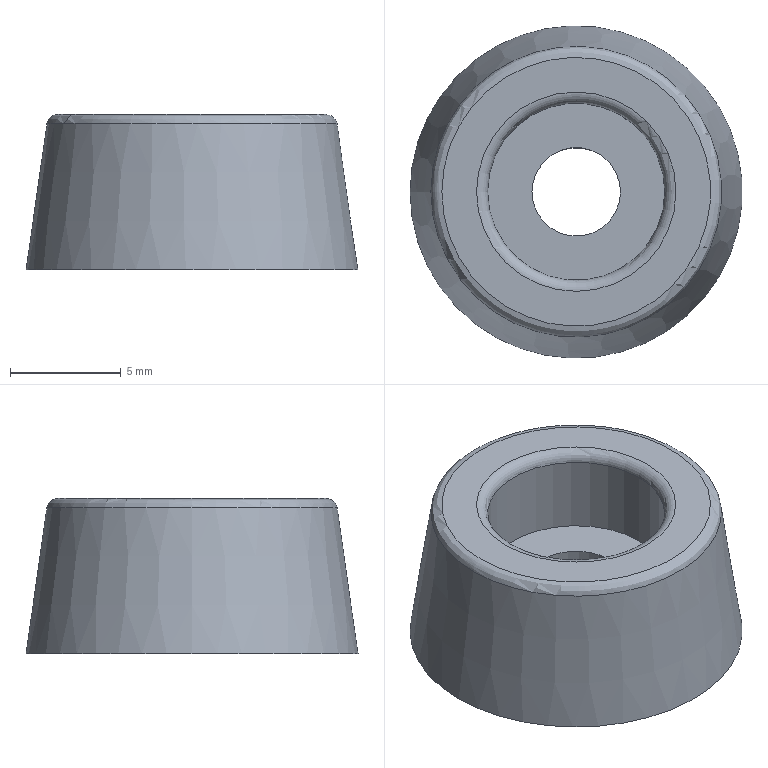Part | NX | 1 solid | 8 faces | box 15 x 15 x 7 mm | volume 837.711 mm3 | plane 3 | cylinder 2 | torus 2 | cone 1 | commonest cylinder face diameters 4 x1 8 x1
STEP:
#1=CARTESIAN_POINT('',(-2.,0.,3.));
#2=VERTEX_POINT('',#1);
#3=CARTESIAN_POINT('',(0.,0.,3.));
#4=DIRECTION('',(0.,0.,-1.));
#5=DIRECTION('',(-1.,0.,0.));
#6=AXIS2_PLACEMENT_3D('',#3,#4,#5);
#7=CIRCLE('',#6,2.);
#8=EDGE_CURVE('',#2,#2,#7,.T.);
#9=ORIENTED_EDGE('',*,*,#8,.F.);
#10=EDGE_LOOP('',(#9));
#11=FACE_BOUND('',#10,.T.);
#12=CARTESIAN_POINT('',(-2.,0.,0.));
#13=VERTEX_POINT('',#12);
#14=CARTESIAN_POINT('',(0.,0.,0.));
#15=DIRECTION('',(0.,0.,-1.));
#16=DIRECTION('',(-1.,0.,0.));
#17=AXIS2_PLACEMENT_3D('',#14,#15,#16);
#18=CIRCLE('',#17,2.);
#19=EDGE_CURVE('',#13,#13,#18,.T.);
#20=ORIENTED_EDGE('',*,*,#19,.T.);
#21=EDGE_LOOP('',(#20));
#22=FACE_BOUND('',#21,.T.);
#23=CARTESIAN_POINT('',(0.,0.,0.));
#24=DIRECTION('',(0.,0.,-1.));
#25=DIRECTION('',(1.,0.,0.));
#26=AXIS2_PLACEMENT_3D('',#23,#24,#25);
#27=CYLINDRICAL_SURFACE('',#26,2.);
#28=ADVANCED_FACE('',(#11,#22),#27,.F.);
#29=CARTESIAN_POINT('',(-4.,0.,3.));
#30=VERTEX_POINT('',#29);
#31=CARTESIAN_POINT('',(0.,0.,3.));
#32=DIRECTION('',(0.,0.,-1.));
#33=DIRECTION('',(-1.,0.,0.));
#34=AXIS2_PLACEMENT_3D('',#31,#32,#33);
#35=CIRCLE('',#34,4.);
#36=EDGE_CURVE('',#30,#30,#35,.T.);
#37=ORIENTED_EDGE('',*,*,#36,.F.);
#38=EDGE_LOOP('',(#37));
#39=FACE_BOUND('',#38,.T.);
#40=ORIENTED_EDGE('',*,*,#8,.T.);
#41=EDGE_LOOP('',(#40));
#42=FACE_BOUND('',#41,.T.);
#43=CARTESIAN_POINT('',(0.,2.,3.));
#44=DIRECTION('',(0.,0.,-1.));
#45=DIRECTION('',(1.,0.,0.));
#46=AXIS2_PLACEMENT_3D('',#43,#44,#45);
#47=PLANE('',#46);
#48=ADVANCED_FACE('',(#39,#42),#47,.F.);
#49=CARTESIAN_POINT('',(-4.,0.,6.5));
#50=VERTEX_POINT('',#49);
#51=CARTESIAN_POINT('',(0.,0.,6.5));
#52=DIRECTION('',(0.,0.,-1.));
#53=DIRECTION('',(-1.,0.,0.));
#54=AXIS2_PLACEMENT_3D('',#51,#52,#53);
#55=CIRCLE('',#54,4.);
#56=EDGE_CURVE('',#50,#50,#55,.T.);
#57=ORIENTED_EDGE('',*,*,#56,.F.);
#58=EDGE_LOOP('',(#57));
#59=FACE_BOUND('',#58,.T.);
#60=ORIENTED_EDGE('',*,*,#36,.T.);
#61=EDGE_LOOP('',(#60));
#62=FACE_BOUND('',#61,.T.);
#63=CARTESIAN_POINT('',(0.,0.,0.));
#64=DIRECTION('',(0.,0.,-1.));
#65=DIRECTION('',(1.,0.,0.));
#66=AXIS2_PLACEMENT_3D('',#63,#64,#65);
#67=CYLINDRICAL_SURFACE('',#66,4.);
#68=ADVANCED_FACE('',(#59,#62),#67,.F.);
#69=CARTESIAN_POINT('',(-4.5,0.,7.));
#70=VERTEX_POINT('',#69);
#71=CARTESIAN_POINT('',(0.,0.,7.));
#72=DIRECTION('',(0.,0.,-1.));
#73=DIRECTION('',(-1.,0.,0.));
#74=AXIS2_PLACEMENT_3D('',#71,#72,#73);
#75=CIRCLE('',#74,4.5);
#76=EDGE_CURVE('',#70,#70,#75,.T.);
#77=ORIENTED_EDGE('',*,*,#76,.F.);
#78=EDGE_LOOP('',(#77));
#79=FACE_BOUND('',#78,.T.);
#80=ORIENTED_EDGE('',*,*,#56,.T.);
#81=EDGE_LOOP('',(#80));
#82=FACE_BOUND('',#81,.T.);
#83=CARTESIAN_POINT('',(0.,0.,6.5));
#84=DIRECTION('',(0.,0.,-1.));
#85=DIRECTION('',(1.,0.,0.));
#86=AXIS2_PLACEMENT_3D('',#83,#84,#85);
#87=TOROIDAL_SURFACE('',#86,4.5,0.5);
#88=ADVANCED_FACE('',(#79,#82),#87,.T.);
#89=CARTESIAN_POINT('',(-6.066,0.,7.));
#90=VERTEX_POINT('',#89);
#91=CARTESIAN_POINT('',(0.,0.,7.));
#92=DIRECTION('',(0.,0.,-1.));
#93=DIRECTION('',(-1.,0.,0.));
#94=AXIS2_PLACEMENT_3D('',#91,#92,#93);
#95=CIRCLE('',#94,6.066);
#96=EDGE_CURVE('',#90,#90,#95,.T.);
#97=ORIENTED_EDGE('',*,*,#96,.F.);
#98=EDGE_LOOP('',(#97));
#99=FACE_BOUND('',#98,.T.);
#100=ORIENTED_EDGE('',*,*,#76,.T.);
#101=EDGE_LOOP('',(#100));
#102=FACE_BOUND('',#101,.T.);
#103=CARTESIAN_POINT('',(0.,4.5,7.));
#104=DIRECTION('',(0.,0.,-1.));
#105=DIRECTION('',(1.,0.,0.));
#106=AXIS2_PLACEMENT_3D('',#103,#104,#105);
#107=PLANE('',#106);
#108=ADVANCED_FACE('',(#99,#102),#107,.F.);
#109=CARTESIAN_POINT('',(-6.561,0.,6.571));
#110=VERTEX_POINT('',#109);
#111=CARTESIAN_POINT('',(0.,0.,6.571));
#112=DIRECTION('',(0.,0.,-1.));
#113=DIRECTION('',(-1.,0.,0.));
#114=AXIS2_PLACEMENT_3D('',#111,#112,#113);
#115=CIRCLE('',#114,6.561);
#116=EDGE_CURVE('',#110,#110,#115,.T.);
#117=ORIENTED_EDGE('',*,*,#116,.F.);
#118=EDGE_LOOP('',(#117));
#119=FACE_BOUND('',#118,.T.);
#120=ORIENTED_EDGE('',*,*,#96,.T.);
#121=EDGE_LOOP('',(#120));
#122=FACE_BOUND('',#121,.T.);
#123=CARTESIAN_POINT('',(0.,0.,6.5));
#124=DIRECTION('',(0.,0.,-1.));
#125=DIRECTION('',(1.,0.,0.));
#126=AXIS2_PLACEMENT_3D('',#123,#124,#125);
#127=TOROIDAL_SURFACE('',#126,6.066,0.5);
#128=ADVANCED_FACE('',(#119,#122),#127,.T.);
#129=CARTESIAN_POINT('',(-7.5,0.,0.));
#130=VERTEX_POINT('',#129);
#131=CARTESIAN_POINT('',(0.,0.,0.));
#132=DIRECTION('',(0.,0.,-1.));
#133=DIRECTION('',(-1.,0.,0.));
#134=AXIS2_PLACEMENT_3D('',#131,#132,#133);
#135=CIRCLE('',#134,7.5);
#136=EDGE_CURVE('',#130,#130,#135,.T.);
#137=ORIENTED_EDGE('',*,*,#136,.F.);
#138=EDGE_LOOP('',(#137));
#139=FACE_BOUND('',#138,.T.);
#140=ORIENTED_EDGE('',*,*,#116,.T.);
#141=EDGE_LOOP('',(#140));
#142=FACE_BOUND('',#141,.T.);
#143=CARTESIAN_POINT('',(0.,0.,6.571));
#144=DIRECTION('',(0.,0.,-1.));
#145=DIRECTION('',(1.,0.,0.));
#146=AXIS2_PLACEMENT_3D('',#143,#144,#145);
#147=CONICAL_SURFACE('',#146,6.561,8.13);
#148=ADVANCED_FACE('',(#139,#142),#147,.T.);
#149=ORIENTED_EDGE('',*,*,#19,.F.);
#150=EDGE_LOOP('',(#149));
#151=FACE_BOUND('',#150,.T.);
#152=ORIENTED_EDGE('',*,*,#136,.T.);
#153=EDGE_LOOP('',(#152));
#154=FACE_BOUND('',#153,.T.);
#155=CARTESIAN_POINT('',(0.,7.5,0.));
#156=DIRECTION('',(0.,0.,1.));
#157=DIRECTION('',(-1.,0.,0.));
#158=AXIS2_PLACEMENT_3D('',#155,#156,#157);
#159=PLANE('',#158);
#160=ADVANCED_FACE('',(#151,#154),#159,.F.);
#161=CLOSED_SHELL('',(#28,#48,#68,#88,#108,#128,#148,#160));
#162=MANIFOLD_SOLID_BREP('',#161);
#163=(LENGTH_UNIT()NAMED_UNIT(*)SI_UNIT(.MILLI.,.METRE.));
#164=UNCERTAINTY_MEASURE_WITH_UNIT(LENGTH_MEASURE(0.00002),#163,'','');
#165=(NAMED_UNIT(*)PLANE_ANGLE_UNIT()SI_UNIT($,.RADIAN.));
#166=PLANE_ANGLE_MEASURE_WITH_UNIT(PLANE_ANGLE_MEASURE(0.01745),#165);
#167=DIMENSIONAL_EXPONENTS(0.,0.,0.,0.,0.,0.,0.);
#168=(CONVERSION_BASED_UNIT('DEGREE',#166)NAMED_UNIT(#167)PLANE_ANGLE_UNIT());
#169=(NAMED_UNIT(*)SI_UNIT($,.STERADIAN.)SOLID_ANGLE_UNIT());
#170=(GEOMETRIC_REPRESENTATION_CONTEXT(3)GLOBAL_UNCERTAINTY_ASSIGNED_CONTEXT((#164))GLOBAL_UNIT_ASSIGNED_CONTEXT((#163,#168,#169))REPRESENTATION_CONTEXT('',''));
#171=ADVANCED_BREP_SHAPE_REPRESENTATION('',(#162),#170);